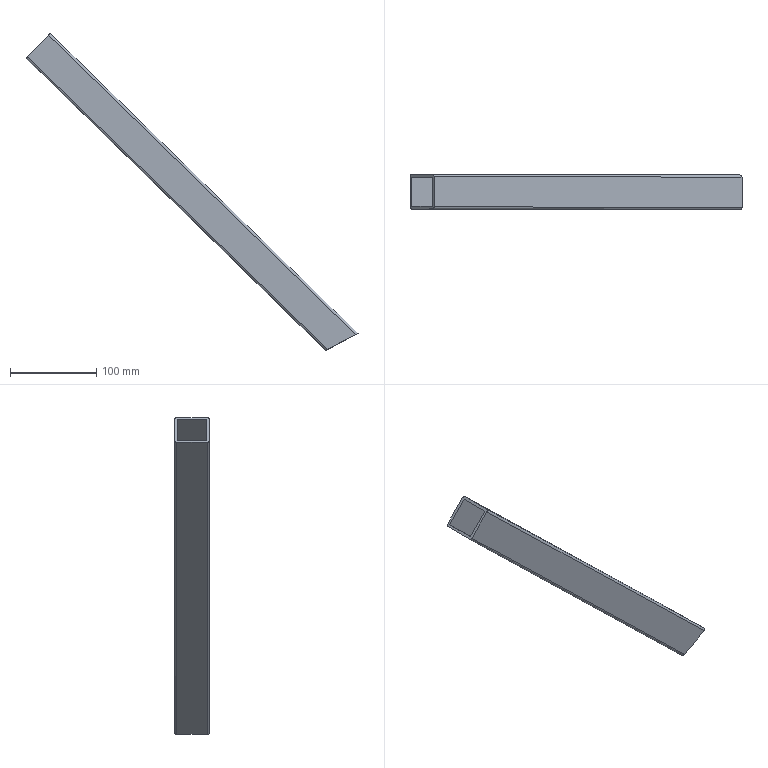Part | STEP file | SOLID | 1 solid | 14 faces | box 384.531 x 40 x 366.951 mm | volume 215519 mm3 | plane 10 | cylinder 4 | commonest cylinder face diameters 5 x4
STEP:
#1=CARTESIAN_POINT('',(0.,0.,0.));
#2=DIRECTION('',(0.,0.,1.));
#3=DIRECTION('',(1.,0.,0.));
#4=AXIS2_PLACEMENT_3D('',#1,#2,#3);
#5=CARTESIAN_POINT('',(1687.954,187.75,-2.424));
#6=VERTEX_POINT('',#5);
#7=CARTESIAN_POINT('',(1711.675,187.75,21.934));
#8=VERTEX_POINT('',#7);
#9=CARTESIAN_POINT('',(867.562,187.75,-844.86));
#10=DIRECTION('',(0.6977,0.,0.7164));
#11=VECTOR('',#10,1.);
#12=LINE('',#9,#11);
#13=CARTESIAN_POINT('',(0.,187.75,0.));
#14=DIRECTION('',(0.,1.,0.));
#15=DIRECTION('',(0.,0.,-1.));
#16=AXIS2_PLACEMENT_3D('',#13,#14,#15);
#17=PLANE('',#16);
#18=CARTESIAN_POINT('',(844.86,-867.562));
#19=DIRECTION('',(-0.7164,-0.6977));
#20=VECTOR('',#19,1.);
#21=LINE('',#18,#20);
#22=(GEOMETRIC_REPRESENTATION_CONTEXT(2)PARAMETRIC_REPRESENTATION_CONTEXT()REPRESENTATION_CONTEXT('',''));
#23=DEFINITIONAL_REPRESENTATION('',(#21),#22);
#24=PCURVE('',#17,#23);
#25=CARTESIAN_POINT('',(1685.861,150.75,-4.573));
#26=DIRECTION('',(-0.7164,0.,0.6977));
#27=DIRECTION('',(-0.6977,0.,-0.7164));
#28=AXIS2_PLACEMENT_3D('',#25,#26,#27);
#29=PLANE('',#28);
#30=CARTESIAN_POINT('',(1172.901,-37.));
#31=DIRECTION('',(-1.,0.));
#32=VECTOR('',#31,1.);
#33=LINE('',#30,#32);
#34=(GEOMETRIC_REPRESENTATION_CONTEXT(2)PARAMETRIC_REPRESENTATION_CONTEXT()REPRESENTATION_CONTEXT('',''));
#35=DEFINITIONAL_REPRESENTATION('',(#33),#34);
#36=PCURVE('',#29,#35);
#37=SURFACE_CURVE('',#12,(#24,#36),.PCURVE_S1.);
#38=EDGE_CURVE('',#6,#8,#37,.T.);
#39=ORIENTED_EDGE('',*,*,#38,.F.);
#40=CARTESIAN_POINT('',(2036.032,187.75,-341.393));
#41=VERTEX_POINT('',#40);
#42=CARTESIAN_POINT('',(2035.339,187.75,-340.718));
#43=DIRECTION('',(0.7164,0.,-0.6977));
#44=VECTOR('',#43,1.);
#45=LINE('',#42,#44);
#46=CARTESIAN_POINT('',(340.718,-2035.339));
#47=DIRECTION('',(0.6977,-0.7164));
#48=VECTOR('',#47,1.);
#49=LINE('',#46,#48);
#50=(GEOMETRIC_REPRESENTATION_CONTEXT(2)PARAMETRIC_REPRESENTATION_CONTEXT()REPRESENTATION_CONTEXT('',''));
#51=DEFINITIONAL_REPRESENTATION('',(#49),#50);
#52=PCURVE('',#17,#51);
#53=CARTESIAN_POINT('',(2035.339,150.75,-340.718));
#54=DIRECTION('',(-0.6977,0.,-0.7164));
#55=DIRECTION('',(0.7164,0.,-0.6977));
#56=AXIS2_PLACEMENT_3D('',#53,#54,#55);
#57=PLANE('',#56);
#58=CARTESIAN_POINT('',(0.,-37.));
#59=DIRECTION('',(1.,0.));
#60=VECTOR('',#59,1.);
#61=LINE('',#58,#60);
#62=(GEOMETRIC_REPRESENTATION_CONTEXT(2)PARAMETRIC_REPRESENTATION_CONTEXT()REPRESENTATION_CONTEXT('',''));
#63=DEFINITIONAL_REPRESENTATION('',(#61),#62);
#64=PCURVE('',#57,#63);
#65=SURFACE_CURVE('',#45,(#52,#64),.PCURVE_S1.);
#66=EDGE_CURVE('',#6,#41,#65,.T.);
#67=ORIENTED_EDGE('',*,*,#66,.T.);
#68=CARTESIAN_POINT('',(2067.606,187.75,-324.683));
#69=VERTEX_POINT('',#68);
#70=CARTESIAN_POINT('',(586.635,187.75,-1108.462));
#71=DIRECTION('',(-0.8839,0.,-0.4678));
#72=VECTOR('',#71,1.);
#73=LINE('',#70,#72);
#74=CARTESIAN_POINT('',(1108.462,-586.635));
#75=DIRECTION('',(0.4678,0.8839));
#76=VECTOR('',#75,1.);
#77=LINE('',#74,#76);
#78=(GEOMETRIC_REPRESENTATION_CONTEXT(2)PARAMETRIC_REPRESENTATION_CONTEXT()REPRESENTATION_CONTEXT('',''));
#79=DEFINITIONAL_REPRESENTATION('',(#77),#78);
#80=PCURVE('',#17,#79);
#81=CARTESIAN_POINT('',(2070.392,150.75,-323.209));
#82=DIRECTION('',(0.4678,0.,-0.8839));
#83=DIRECTION('',(0.8839,0.,0.4678));
#84=AXIS2_PLACEMENT_3D('',#81,#82,#83);
#85=PLANE('',#84);
#86=CARTESIAN_POINT('',(-1678.738,-37.));
#87=DIRECTION('',(-1.,0.));
#88=VECTOR('',#87,1.);
#89=LINE('',#86,#88);
#90=(GEOMETRIC_REPRESENTATION_CONTEXT(2)PARAMETRIC_REPRESENTATION_CONTEXT()REPRESENTATION_CONTEXT('',''));
#91=DEFINITIONAL_REPRESENTATION('',(#89),#90);
#92=PCURVE('',#85,#91);
#93=SURFACE_CURVE('',#73,(#80,#92),.PCURVE_S1.);
#94=EDGE_CURVE('',#69,#41,#93,.T.);
#95=ORIENTED_EDGE('',*,*,#94,.F.);
#96=CARTESIAN_POINT('',(1640.033,187.75,91.702));
#97=DIRECTION('',(-0.7164,0.,0.6977));
#98=VECTOR('',#97,1.);
#99=LINE('',#96,#98);
#100=CARTESIAN_POINT('',(-91.702,-1640.033));
#101=DIRECTION('',(-0.6977,0.7164));
#102=VECTOR('',#101,1.);
#103=LINE('',#100,#102);
#104=(GEOMETRIC_REPRESENTATION_CONTEXT(2)PARAMETRIC_REPRESENTATION_CONTEXT()REPRESENTATION_CONTEXT('',''));
#105=DEFINITIONAL_REPRESENTATION('',(#103),#104);
#106=PCURVE('',#17,#105);
#107=CARTESIAN_POINT('',(1640.033,150.75,91.702));
#108=DIRECTION('',(0.6977,0.,0.7164));
#109=DIRECTION('',(-0.7164,0.,0.6977));
#110=AXIS2_PLACEMENT_3D('',#107,#108,#109);
#111=PLANE('',#110);
#112=CARTESIAN_POINT('',(0.,-37.));
#113=DIRECTION('',(1.,0.));
#114=VECTOR('',#113,1.);
#115=LINE('',#112,#114);
#116=(GEOMETRIC_REPRESENTATION_CONTEXT(2)PARAMETRIC_REPRESENTATION_CONTEXT()REPRESENTATION_CONTEXT('',''));
#117=DEFINITIONAL_REPRESENTATION('',(#115),#116);
#118=PCURVE('',#111,#117);
#119=SURFACE_CURVE('',#99,(#106,#118),.PCURVE_S1.);
#120=EDGE_CURVE('',#69,#8,#119,.T.);
#121=ORIENTED_EDGE('',*,*,#120,.T.);
#122=EDGE_LOOP('',(#39,#67,#95,#121));
#123=FACE_BOUND('',#122,.T.);
#124=ADVANCED_FACE('',(#123),#17,.F.);
#125=CARTESIAN_POINT('',(2067.606,153.75,-324.683));
#126=VERTEX_POINT('',#125);
#127=CARTESIAN_POINT('',(2036.032,153.75,-341.393));
#128=VERTEX_POINT('',#127);
#129=CARTESIAN_POINT('',(586.635,153.75,-1108.462));
#130=DIRECTION('',(-0.8839,0.,-0.4678));
#131=VECTOR('',#130,1.);
#132=LINE('',#129,#131);
#133=CARTESIAN_POINT('',(0.,153.75,0.));
#134=DIRECTION('',(0.,1.,0.));
#135=DIRECTION('',(0.,0.,-1.));
#136=AXIS2_PLACEMENT_3D('',#133,#134,#135);
#137=PLANE('',#136);
#138=CARTESIAN_POINT('',(1108.462,-586.635));
#139=DIRECTION('',(0.4678,0.8839));
#140=VECTOR('',#139,1.);
#141=LINE('',#138,#140);
#142=(GEOMETRIC_REPRESENTATION_CONTEXT(2)PARAMETRIC_REPRESENTATION_CONTEXT()REPRESENTATION_CONTEXT('',''));
#143=DEFINITIONAL_REPRESENTATION('',(#141),#142);
#144=PCURVE('',#137,#143);
#145=CARTESIAN_POINT('',(-1678.738,-3.));
#146=DIRECTION('',(-1.,0.));
#147=VECTOR('',#146,1.);
#148=LINE('',#145,#147);
#149=(GEOMETRIC_REPRESENTATION_CONTEXT(2)PARAMETRIC_REPRESENTATION_CONTEXT()REPRESENTATION_CONTEXT('',''));
#150=DEFINITIONAL_REPRESENTATION('',(#148),#149);
#151=PCURVE('',#85,#150);
#152=SURFACE_CURVE('',#132,(#144,#151),.PCURVE_S1.);
#153=EDGE_CURVE('',#126,#128,#152,.T.);
#154=ORIENTED_EDGE('',*,*,#153,.T.);
#155=CARTESIAN_POINT('',(1687.954,153.75,-2.424));
#156=VERTEX_POINT('',#155);
#157=CARTESIAN_POINT('',(2035.339,153.75,-340.718));
#158=DIRECTION('',(0.7164,0.,-0.6977));
#159=VECTOR('',#158,1.);
#160=LINE('',#157,#159);
#161=CARTESIAN_POINT('',(340.718,-2035.339));
#162=DIRECTION('',(0.6977,-0.7164));
#163=VECTOR('',#162,1.);
#164=LINE('',#161,#163);
#165=(GEOMETRIC_REPRESENTATION_CONTEXT(2)PARAMETRIC_REPRESENTATION_CONTEXT()REPRESENTATION_CONTEXT('',''));
#166=DEFINITIONAL_REPRESENTATION('',(#164),#165);
#167=PCURVE('',#137,#166);
#168=CARTESIAN_POINT('',(0.,-3.));
#169=DIRECTION('',(1.,0.));
#170=VECTOR('',#169,1.);
#171=LINE('',#168,#170);
#172=(GEOMETRIC_REPRESENTATION_CONTEXT(2)PARAMETRIC_REPRESENTATION_CONTEXT()REPRESENTATION_CONTEXT('',''));
#173=DEFINITIONAL_REPRESENTATION('',(#171),#172);
#174=PCURVE('',#57,#173);
#175=SURFACE_CURVE('',#160,(#167,#174),.PCURVE_S1.);
#176=EDGE_CURVE('',#156,#128,#175,.T.);
#177=ORIENTED_EDGE('',*,*,#176,.F.);
#178=CARTESIAN_POINT('',(1711.675,153.75,21.934));
#179=VERTEX_POINT('',#178);
#180=CARTESIAN_POINT('',(867.562,153.75,-844.86));
#181=DIRECTION('',(0.6977,0.,0.7164));
#182=VECTOR('',#181,1.);
#183=LINE('',#180,#182);
#184=CARTESIAN_POINT('',(844.86,-867.562));
#185=DIRECTION('',(-0.7164,-0.6977));
#186=VECTOR('',#185,1.);
#187=LINE('',#184,#186);
#188=(GEOMETRIC_REPRESENTATION_CONTEXT(2)PARAMETRIC_REPRESENTATION_CONTEXT()REPRESENTATION_CONTEXT('',''));
#189=DEFINITIONAL_REPRESENTATION('',(#187),#188);
#190=PCURVE('',#137,#189);
#191=CARTESIAN_POINT('',(1172.901,-3.));
#192=DIRECTION('',(-1.,0.));
#193=VECTOR('',#192,1.);
#194=LINE('',#191,#193);
#195=(GEOMETRIC_REPRESENTATION_CONTEXT(2)PARAMETRIC_REPRESENTATION_CONTEXT()REPRESENTATION_CONTEXT('',''));
#196=DEFINITIONAL_REPRESENTATION('',(#194),#195);
#197=PCURVE('',#29,#196);
#198=SURFACE_CURVE('',#183,(#190,#197),.PCURVE_S1.);
#199=EDGE_CURVE('',#156,#179,#198,.T.);
#200=ORIENTED_EDGE('',*,*,#199,.T.);
#201=CARTESIAN_POINT('',(1640.033,153.75,91.702));
#202=DIRECTION('',(-0.7164,0.,0.6977));
#203=VECTOR('',#202,1.);
#204=LINE('',#201,#203);
#205=CARTESIAN_POINT('',(-91.702,-1640.033));
#206=DIRECTION('',(-0.6977,0.7164));
#207=VECTOR('',#206,1.);
#208=LINE('',#205,#207);
#209=(GEOMETRIC_REPRESENTATION_CONTEXT(2)PARAMETRIC_REPRESENTATION_CONTEXT()REPRESENTATION_CONTEXT('',''));
#210=DEFINITIONAL_REPRESENTATION('',(#208),#209);
#211=PCURVE('',#137,#210);
#212=CARTESIAN_POINT('',(0.,-3.));
#213=DIRECTION('',(1.,0.));
#214=VECTOR('',#213,1.);
#215=LINE('',#212,#214);
#216=(GEOMETRIC_REPRESENTATION_CONTEXT(2)PARAMETRIC_REPRESENTATION_CONTEXT()REPRESENTATION_CONTEXT('',''));
#217=DEFINITIONAL_REPRESENTATION('',(#215),#216);
#218=PCURVE('',#111,#217);
#219=SURFACE_CURVE('',#204,(#211,#218),.PCURVE_S1.);
#220=EDGE_CURVE('',#126,#179,#219,.T.);
#221=ORIENTED_EDGE('',*,*,#220,.F.);
#222=EDGE_LOOP('',(#154,#177,#200,#221));
#223=FACE_BOUND('',#222,.T.);
#224=ADVANCED_FACE('',(#223),#137,.T.);
#225=CARTESIAN_POINT('',(1711.675,150.75,21.934));
#226=DIRECTION('',(0.,1.,0.));
#227=VECTOR('',#226,1.);
#228=LINE('',#225,#227);
#229=CARTESIAN_POINT('',(-100.,0.));
#230=DIRECTION('',(0.,-1.));
#231=VECTOR('',#230,1.);
#232=LINE('',#229,#231);
#233=(GEOMETRIC_REPRESENTATION_CONTEXT(2)PARAMETRIC_REPRESENTATION_CONTEXT()REPRESENTATION_CONTEXT('',''));
#234=DEFINITIONAL_REPRESENTATION('',(#232),#233);
#235=PCURVE('',#111,#234);
#236=CARTESIAN_POINT('',(-37.,0.));
#237=DIRECTION('',(0.,-1.));
#238=VECTOR('',#237,1.);
#239=LINE('',#236,#238);
#240=(GEOMETRIC_REPRESENTATION_CONTEXT(2)PARAMETRIC_REPRESENTATION_CONTEXT()REPRESENTATION_CONTEXT('',''));
#241=DEFINITIONAL_REPRESENTATION('',(#239),#240);
#242=PCURVE('',#29,#241);
#243=SURFACE_CURVE('',#228,(#235,#242),.PCURVE_S1.);
#244=EDGE_CURVE('',#179,#8,#243,.T.);
#245=ORIENTED_EDGE('',*,*,#244,.T.);
#246=ORIENTED_EDGE('',*,*,#120,.F.);
#247=CARTESIAN_POINT('',(2067.606,150.75,-324.683));
#248=DIRECTION('',(0.,1.,0.));
#249=VECTOR('',#248,1.);
#250=LINE('',#247,#249);
#251=CARTESIAN_POINT('',(-596.821,0.));
#252=DIRECTION('',(0.,-1.));
#253=VECTOR('',#252,1.);
#254=LINE('',#251,#253);
#255=(GEOMETRIC_REPRESENTATION_CONTEXT(2)PARAMETRIC_REPRESENTATION_CONTEXT()REPRESENTATION_CONTEXT('',''));
#256=DEFINITIONAL_REPRESENTATION('',(#254),#255);
#257=PCURVE('',#111,#256);
#258=CARTESIAN_POINT('',(-3.152,0.));
#259=DIRECTION('',(0.,-1.));
#260=VECTOR('',#259,1.);
#261=LINE('',#258,#260);
#262=(GEOMETRIC_REPRESENTATION_CONTEXT(2)PARAMETRIC_REPRESENTATION_CONTEXT()REPRESENTATION_CONTEXT('',''));
#263=DEFINITIONAL_REPRESENTATION('',(#261),#262);
#264=PCURVE('',#85,#263);
#265=SURFACE_CURVE('',#250,(#257,#264),.PCURVE_S1.);
#266=EDGE_CURVE('',#126,#69,#265,.T.);
#267=ORIENTED_EDGE('',*,*,#266,.F.);
#268=ORIENTED_EDGE('',*,*,#220,.T.);
#269=EDGE_LOOP('',(#245,#246,#267,#268));
#270=FACE_BOUND('',#269,.T.);
#271=ADVANCED_FACE('',(#270),#111,.F.);
#272=CARTESIAN_POINT('',(2036.032,150.75,-341.393));
#273=DIRECTION('',(0.,1.,0.));
#274=VECTOR('',#273,1.);
#275=LINE('',#272,#274);
#276=CARTESIAN_POINT('',(0.9673,0.));
#277=DIRECTION('',(0.,-1.));
#278=VECTOR('',#277,1.);
#279=LINE('',#276,#278);
#280=(GEOMETRIC_REPRESENTATION_CONTEXT(2)PARAMETRIC_REPRESENTATION_CONTEXT()REPRESENTATION_CONTEXT('',''));
#281=DEFINITIONAL_REPRESENTATION('',(#279),#280);
#282=PCURVE('',#57,#281);
#283=CARTESIAN_POINT('',(-38.876,0.));
#284=DIRECTION('',(0.,-1.));
#285=VECTOR('',#284,1.);
#286=LINE('',#283,#285);
#287=(GEOMETRIC_REPRESENTATION_CONTEXT(2)PARAMETRIC_REPRESENTATION_CONTEXT()REPRESENTATION_CONTEXT('',''));
#288=DEFINITIONAL_REPRESENTATION('',(#286),#287);
#289=PCURVE('',#85,#288);
#290=SURFACE_CURVE('',#275,(#282,#289),.PCURVE_S1.);
#291=EDGE_CURVE('',#128,#41,#290,.T.);
#292=ORIENTED_EDGE('',*,*,#291,.T.);
#293=ORIENTED_EDGE('',*,*,#66,.F.);
#294=CARTESIAN_POINT('',(1687.954,150.75,-2.424));
#295=DIRECTION('',(0.,1.,0.));
#296=VECTOR('',#295,1.);
#297=LINE('',#294,#296);
#298=CARTESIAN_POINT('',(-484.891,0.));
#299=DIRECTION('',(0.,-1.));
#300=VECTOR('',#299,1.);
#301=LINE('',#298,#300);
#302=(GEOMETRIC_REPRESENTATION_CONTEXT(2)PARAMETRIC_REPRESENTATION_CONTEXT()REPRESENTATION_CONTEXT('',''));
#303=DEFINITIONAL_REPRESENTATION('',(#301),#302);
#304=PCURVE('',#57,#303);
#305=CARTESIAN_POINT('',(-3.,0.));
#306=DIRECTION('',(0.,-1.));
#307=VECTOR('',#306,1.);
#308=LINE('',#305,#307);
#309=(GEOMETRIC_REPRESENTATION_CONTEXT(2)PARAMETRIC_REPRESENTATION_CONTEXT()REPRESENTATION_CONTEXT('',''));
#310=DEFINITIONAL_REPRESENTATION('',(#308),#309);
#311=PCURVE('',#29,#310);
#312=SURFACE_CURVE('',#297,(#304,#311),.PCURVE_S1.);
#313=EDGE_CURVE('',#156,#6,#312,.T.);
#314=ORIENTED_EDGE('',*,*,#313,.F.);
#315=ORIENTED_EDGE('',*,*,#176,.T.);
#316=EDGE_LOOP('',(#292,#293,#314,#315));
#317=FACE_BOUND('',#316,.T.);
#318=ADVANCED_FACE('',(#317),#57,.F.);
#319=CARTESIAN_POINT('',(2033.246,188.25,-342.868));
#320=VERTEX_POINT('',#319);
#321=CARTESIAN_POINT('',(2035.568,190.75,-341.639));
#322=VERTEX_POINT('',#321);
#323=CARTESIAN_POINT('',(2035.568,188.25,-341.639));
#324=DIRECTION('',(0.4678,0.,-0.8839));
#325=DIRECTION('',(-0.8839,0.,-0.4678));
#326=AXIS2_PLACEMENT_3D('',#323,#324,#325);
#327=ELLIPSE('',#326,2.627,2.5);
#328=CARTESIAN_POINT('',(820.043,188.25,842.078));
#329=DIRECTION('',(-0.7164,0.,0.6977));
#330=DIRECTION('',(-0.6977,0.,-0.7164));
#331=AXIS2_PLACEMENT_3D('',#328,#329,#330);
#332=CYLINDRICAL_SURFACE('',#331,2.5);
#333=CARTESIAN_POINT('',(6.283,-1695.863));
#334=CARTESIAN_POINT('',(6.259,-1695.863));
#335=CARTESIAN_POINT('',(6.212,-1695.865));
#336=CARTESIAN_POINT('',(6.14,-1695.871));
#337=CARTESIAN_POINT('',(6.069,-1695.881));
#338=CARTESIAN_POINT('',(5.998,-1695.895));
#339=CARTESIAN_POINT('',(5.926,-1695.913));
#340=CARTESIAN_POINT('',(5.855,-1695.935));
#341=CARTESIAN_POINT('',(5.783,-1695.961));
#342=CARTESIAN_POINT('',(5.712,-1695.991));
#343=CARTESIAN_POINT('',(5.641,-1696.023));
#344=CARTESIAN_POINT('',(5.569,-1696.06));
#345=CARTESIAN_POINT('',(5.498,-1696.099));
#346=CARTESIAN_POINT('',(5.426,-1696.141));
#347=CARTESIAN_POINT('',(5.355,-1696.186));
#348=CARTESIAN_POINT('',(5.284,-1696.233));
#349=CARTESIAN_POINT('',(5.212,-1696.283));
#350=CARTESIAN_POINT('',(5.141,-1696.334));
#351=CARTESIAN_POINT('',(5.069,-1696.387));
#352=CARTESIAN_POINT('',(4.998,-1696.442));
#353=CARTESIAN_POINT('',(4.927,-1696.498));
#354=CARTESIAN_POINT('',(4.855,-1696.554));
#355=CARTESIAN_POINT('',(4.784,-1696.612));
#356=CARTESIAN_POINT('',(4.736,-1696.65));
#357=CARTESIAN_POINT('',(4.712,-1696.669));
#358=B_SPLINE_CURVE_WITH_KNOTS('',3,(#333,#334,#335,#336,#337,#338,#339,#340,#341,#342,#343,#344,#345,#346,#347,#348,#349,#350,#351,#352,#353,#354,#355,#356,#357),.UNSPECIFIED.,.F.,.F.,(4,1,1,1,1,1,1,1,1,1,1,1,1,1,1,1,1,1,1,1,1,1,4),(0.,0.0714,0.1428,0.2142,0.2856,0.357,0.4284,0.4998,0.5712,0.6426,0.714,0.7854,0.8568,0.9282,0.9996,1.071,1.142,1.214,1.285,1.357,1.428,1.499,1.571),.QUASI_UNIFORM_KNOTS.);
#359=(GEOMETRIC_REPRESENTATION_CONTEXT(2)PARAMETRIC_REPRESENTATION_CONTEXT()REPRESENTATION_CONTEXT('',''));
#360=DEFINITIONAL_REPRESENTATION('',(#358),#359);
#361=PCURVE('',#332,#360);
#362=CARTESIAN_POINT('',(-39.401,-37.5));
#363=DIRECTION('',(-1.,0.));
#364=AXIS2_PLACEMENT_2D('',#362,#363);
#365=ELLIPSE('',#364,2.627,2.5);
#366=(GEOMETRIC_REPRESENTATION_CONTEXT(2)PARAMETRIC_REPRESENTATION_CONTEXT()REPRESENTATION_CONTEXT('',''));
#367=DEFINITIONAL_REPRESENTATION('',(#365),#366);
#368=PCURVE('',#85,#367);
#369=SURFACE_CURVE('',#327,(#361,#368),.PCURVE_S1.);
#370=EDGE_CURVE('',#320,#322,#369,.T.);
#371=ORIENTED_EDGE('',*,*,#370,.F.);
#372=CARTESIAN_POINT('',(1685.861,188.25,-4.573));
#373=VERTEX_POINT('',#372);
#374=CARTESIAN_POINT('',(2033.246,188.25,-342.868));
#375=DIRECTION('',(0.7164,0.,-0.6977));
#376=VECTOR('',#375,1.);
#377=LINE('',#374,#376);
#378=CARTESIAN_POINT('',(6.283,-1695.863));
#379=DIRECTION('',(0.,-1.));
#380=VECTOR('',#379,1.);
#381=LINE('',#378,#380);
#382=(GEOMETRIC_REPRESENTATION_CONTEXT(2)PARAMETRIC_REPRESENTATION_CONTEXT()REPRESENTATION_CONTEXT('',''));
#383=DEFINITIONAL_REPRESENTATION('',(#381),#382);
#384=PCURVE('',#332,#383);
#385=CARTESIAN_POINT('',(2033.246,150.75,-342.868));
#386=DIRECTION('',(-0.6977,0.,-0.7164));
#387=DIRECTION('',(0.7164,0.,-0.6977));
#388=AXIS2_PLACEMENT_3D('',#385,#386,#387);
#389=PLANE('',#388);
#390=CARTESIAN_POINT('',(0.,-37.5));
#391=DIRECTION('',(1.,0.));
#392=VECTOR('',#391,1.);
#393=LINE('',#390,#392);
#394=(GEOMETRIC_REPRESENTATION_CONTEXT(2)PARAMETRIC_REPRESENTATION_CONTEXT()REPRESENTATION_CONTEXT('',''));
#395=DEFINITIONAL_REPRESENTATION('',(#393),#394);
#396=PCURVE('',#389,#395);
#397=SURFACE_CURVE('',#377,(#384,#396),.PCURVE_S1.);
#398=EDGE_CURVE('',#373,#320,#397,.T.);
#399=ORIENTED_EDGE('',*,*,#398,.F.);
#400=CARTESIAN_POINT('',(1687.606,190.75,-2.782));
#401=VERTEX_POINT('',#400);
#402=CARTESIAN_POINT('',(1687.606,188.25,-2.782));
#403=DIRECTION('',(-0.7164,0.,0.6977));
#404=DIRECTION('',(0.6977,0.,0.7164));
#405=AXIS2_PLACEMENT_3D('',#402,#403,#404);
#406=CIRCLE('',#405,2.5);
#407=CARTESIAN_POINT('',(3.142,-1210.972));
#408=DIRECTION('',(1.,0.));
#409=VECTOR('',#408,1.);
#410=LINE('',#407,#409);
#411=(GEOMETRIC_REPRESENTATION_CONTEXT(2)PARAMETRIC_REPRESENTATION_CONTEXT()REPRESENTATION_CONTEXT('',''));
#412=DEFINITIONAL_REPRESENTATION('',(#410),#411);
#413=PCURVE('',#332,#412);
#414=CARTESIAN_POINT('',(-2.5,-37.5));
#415=DIRECTION('',(-1.,0.));
#416=AXIS2_PLACEMENT_2D('',#414,#415);
#417=CIRCLE('',#416,2.5);
#418=(GEOMETRIC_REPRESENTATION_CONTEXT(2)PARAMETRIC_REPRESENTATION_CONTEXT()REPRESENTATION_CONTEXT('',''));
#419=DEFINITIONAL_REPRESENTATION('',(#417),#418);
#420=PCURVE('',#29,#419);
#421=SURFACE_CURVE('',#406,(#413,#420),.PCURVE_S1.);
#422=EDGE_CURVE('',#401,#373,#421,.T.);
#423=ORIENTED_EDGE('',*,*,#422,.F.);
#424=CARTESIAN_POINT('',(820.043,190.75,842.078));
#425=DIRECTION('',(-0.7164,0.,0.6977));
#426=VECTOR('',#425,1.);
#427=LINE('',#424,#426);
#428=CARTESIAN_POINT('',(4.712,0.));
#429=DIRECTION('',(0.,1.));
#430=VECTOR('',#429,1.);
#431=LINE('',#428,#430);
#432=(GEOMETRIC_REPRESENTATION_CONTEXT(2)PARAMETRIC_REPRESENTATION_CONTEXT()REPRESENTATION_CONTEXT('',''));
#433=DEFINITIONAL_REPRESENTATION('',(#431),#432);
#434=PCURVE('',#332,#433);
#435=CARTESIAN_POINT('',(0.,190.75,0.));
#436=DIRECTION('',(0.,1.,0.));
#437=DIRECTION('',(0.,0.,-1.));
#438=AXIS2_PLACEMENT_3D('',#435,#436,#437);
#439=PLANE('',#438);
#440=CARTESIAN_POINT('',(-842.078,-820.043));
#441=DIRECTION('',(-0.6977,0.7164));
#442=VECTOR('',#441,1.);
#443=LINE('',#440,#442);
#444=(GEOMETRIC_REPRESENTATION_CONTEXT(2)PARAMETRIC_REPRESENTATION_CONTEXT()REPRESENTATION_CONTEXT('',''));
#445=DEFINITIONAL_REPRESENTATION('',(#443),#444);
#446=PCURVE('',#439,#445);
#447=SURFACE_CURVE('',#427,(#434,#446),.PCURVE_S1.);
#448=EDGE_CURVE('',#322,#401,#447,.T.);
#449=ORIENTED_EDGE('',*,*,#448,.F.);
#450=EDGE_LOOP('',(#371,#399,#423,#449));
#451=FACE_BOUND('',#450,.T.);
#452=ADVANCED_FACE('',(#451),#332,.T.);
#453=CARTESIAN_POINT('',(2035.568,150.75,-341.639));
#454=VERTEX_POINT('',#453);
#455=CARTESIAN_POINT('',(2033.246,153.25,-342.868));
#456=VERTEX_POINT('',#455);
#457=CARTESIAN_POINT('',(2035.568,153.25,-341.639));
#458=DIRECTION('',(0.4678,0.,-0.8839));
#459=DIRECTION('',(0.8839,0.,0.4678));
#460=AXIS2_PLACEMENT_3D('',#457,#458,#459);
#461=ELLIPSE('',#460,2.627,2.5);
#462=CARTESIAN_POINT('',(2034.99,153.25,-341.077));
#463=DIRECTION('',(0.7164,0.,-0.6977));
#464=DIRECTION('',(0.6977,0.,0.7164));
#465=AXIS2_PLACEMENT_3D('',#462,#463,#464);
#466=CYLINDRICAL_SURFACE('',#465,2.5);
#467=CARTESIAN_POINT('',(1.571,0.806));
#468=CARTESIAN_POINT('',(1.595,0.7869));
#469=CARTESIAN_POINT('',(1.642,0.7485));
#470=CARTESIAN_POINT('',(1.714,0.6912));
#471=CARTESIAN_POINT('',(1.785,0.6346));
#472=CARTESIAN_POINT('',(1.856,0.5788));
#473=CARTESIAN_POINT('',(1.928,0.5241));
#474=CARTESIAN_POINT('',(1.999,0.4709));
#475=CARTESIAN_POINT('',(2.071,0.4194));
#476=CARTESIAN_POINT('',(2.142,0.3699));
#477=CARTESIAN_POINT('',(2.213,0.3226));
#478=CARTESIAN_POINT('',(2.285,0.2777));
#479=CARTESIAN_POINT('',(2.356,0.2356));
#480=CARTESIAN_POINT('',(2.428,0.1964));
#481=CARTESIAN_POINT('',(2.499,0.1602));
#482=CARTESIAN_POINT('',(2.57,0.1274));
#483=CARTESIAN_POINT('',(2.642,0.098));
#484=CARTESIAN_POINT('',(2.713,0.07222));
#485=CARTESIAN_POINT('',(2.785,0.05018));
#486=CARTESIAN_POINT('',(2.856,0.03199));
#487=CARTESIAN_POINT('',(2.927,0.01775));
#488=CARTESIAN_POINT('',(2.999,0.007526));
#489=CARTESIAN_POINT('',(3.07,0.001371));
#490=CARTESIAN_POINT('',(3.118,-0.000001738));
#491=CARTESIAN_POINT('',(3.142,0.));
#492=B_SPLINE_CURVE_WITH_KNOTS('',3,(#467,#468,#469,#470,#471,#472,#473,#474,#475,#476,#477,#478,#479,#480,#481,#482,#483,#484,#485,#486,#487,#488,#489,#490,#491),.UNSPECIFIED.,.F.,.F.,(4,1,1,1,1,1,1,1,1,1,1,1,1,1,1,1,1,1,1,1,1,1,4),(1.571,1.642,1.714,1.785,1.856,1.928,1.999,2.071,2.142,2.213,2.285,2.356,2.428,2.499,2.57,2.642,2.713,2.785,2.856,2.927,2.999,3.07,3.142),.QUASI_UNIFORM_KNOTS.);
#493=(GEOMETRIC_REPRESENTATION_CONTEXT(2)PARAMETRIC_REPRESENTATION_CONTEXT()REPRESENTATION_CONTEXT('',''));
#494=DEFINITIONAL_REPRESENTATION('',(#492),#493);
#495=PCURVE('',#466,#494);
#496=CARTESIAN_POINT('',(-39.401,-2.5));
#497=DIRECTION('',(1.,0.));
#498=AXIS2_PLACEMENT_2D('',#496,#497);
#499=ELLIPSE('',#498,2.627,2.5);
#500=(GEOMETRIC_REPRESENTATION_CONTEXT(2)PARAMETRIC_REPRESENTATION_CONTEXT()REPRESENTATION_CONTEXT('',''));
#501=DEFINITIONAL_REPRESENTATION('',(#499),#500);
#502=PCURVE('',#85,#501);
#503=SURFACE_CURVE('',#461,(#495,#502),.PCURVE_S1.);
#504=EDGE_CURVE('',#454,#456,#503,.T.);
#505=ORIENTED_EDGE('',*,*,#504,.F.);
#506=CARTESIAN_POINT('',(1687.606,150.75,-2.782));
#507=VERTEX_POINT('',#506);
#508=CARTESIAN_POINT('',(2034.99,150.75,-341.077));
#509=DIRECTION('',(0.7164,0.,-0.6977));
#510=VECTOR('',#509,1.);
#511=LINE('',#508,#510);
#512=CARTESIAN_POINT('',(1.571,0.));
#513=DIRECTION('',(0.,1.));
#514=VECTOR('',#513,1.);
#515=LINE('',#512,#514);
#516=(GEOMETRIC_REPRESENTATION_CONTEXT(2)PARAMETRIC_REPRESENTATION_CONTEXT()REPRESENTATION_CONTEXT('',''));
#517=DEFINITIONAL_REPRESENTATION('',(#515),#516);
#518=PCURVE('',#466,#517);
#519=CARTESIAN_POINT('',(0.,150.75,0.));
#520=DIRECTION('',(0.,1.,0.));
#521=DIRECTION('',(0.,0.,-1.));
#522=AXIS2_PLACEMENT_3D('',#519,#520,#521);
#523=PLANE('',#522);
#524=CARTESIAN_POINT('',(341.077,-2034.99));
#525=DIRECTION('',(0.6977,-0.7164));
#526=VECTOR('',#525,1.);
#527=LINE('',#524,#526);
#528=(GEOMETRIC_REPRESENTATION_CONTEXT(2)PARAMETRIC_REPRESENTATION_CONTEXT()REPRESENTATION_CONTEXT('',''));
#529=DEFINITIONAL_REPRESENTATION('',(#527),#528);
#530=PCURVE('',#523,#529);
#531=SURFACE_CURVE('',#511,(#518,#530),.PCURVE_S1.);
#532=EDGE_CURVE('',#507,#454,#531,.T.);
#533=ORIENTED_EDGE('',*,*,#532,.F.);
#534=CARTESIAN_POINT('',(1685.861,153.25,-4.573));
#535=VERTEX_POINT('',#534);
#536=CARTESIAN_POINT('',(1687.606,153.25,-2.782));
#537=DIRECTION('',(-0.7164,0.,0.6977));
#538=DIRECTION('',(0.6977,0.,0.7164));
#539=AXIS2_PLACEMENT_3D('',#536,#537,#538);
#540=CIRCLE('',#539,2.5);
#541=CARTESIAN_POINT('',(6.283,-484.891));
#542=DIRECTION('',(-1.,0.));
#543=VECTOR('',#542,1.);
#544=LINE('',#541,#543);
#545=(GEOMETRIC_REPRESENTATION_CONTEXT(2)PARAMETRIC_REPRESENTATION_CONTEXT()REPRESENTATION_CONTEXT('',''));
#546=DEFINITIONAL_REPRESENTATION('',(#544),#545);
#547=PCURVE('',#466,#546);
#548=CARTESIAN_POINT('',(-2.5,-2.5));
#549=DIRECTION('',(-1.,0.));
#550=AXIS2_PLACEMENT_2D('',#548,#549);
#551=CIRCLE('',#550,2.5);
#552=(GEOMETRIC_REPRESENTATION_CONTEXT(2)PARAMETRIC_REPRESENTATION_CONTEXT()REPRESENTATION_CONTEXT('',''));
#553=DEFINITIONAL_REPRESENTATION('',(#551),#552);
#554=PCURVE('',#29,#553);
#555=SURFACE_CURVE('',#540,(#547,#554),.PCURVE_S1.);
#556=EDGE_CURVE('',#535,#507,#555,.T.);
#557=ORIENTED_EDGE('',*,*,#556,.F.);
#558=CARTESIAN_POINT('',(1614.22,153.25,65.194));
#559=DIRECTION('',(-0.7164,0.,0.6977));
#560=VECTOR('',#559,1.);
#561=LINE('',#558,#560);
#562=CARTESIAN_POINT('',(3.142,-584.891));
#563=DIRECTION('',(0.,-1.));
#564=VECTOR('',#563,1.);
#565=LINE('',#562,#564);
#566=(GEOMETRIC_REPRESENTATION_CONTEXT(2)PARAMETRIC_REPRESENTATION_CONTEXT()REPRESENTATION_CONTEXT('',''));
#567=DEFINITIONAL_REPRESENTATION('',(#565),#566);
#568=PCURVE('',#466,#567);
#569=CARTESIAN_POINT('',(-584.891,-2.5));
#570=DIRECTION('',(-1.,0.));
#571=VECTOR('',#570,1.);
#572=LINE('',#569,#571);
#573=(GEOMETRIC_REPRESENTATION_CONTEXT(2)PARAMETRIC_REPRESENTATION_CONTEXT()REPRESENTATION_CONTEXT('',''));
#574=DEFINITIONAL_REPRESENTATION('',(#572),#573);
#575=PCURVE('',#389,#574);
#576=SURFACE_CURVE('',#561,(#568,#575),.PCURVE_S1.);
#577=EDGE_CURVE('',#456,#535,#576,.T.);
#578=ORIENTED_EDGE('',*,*,#577,.F.);
#579=EDGE_LOOP('',(#505,#533,#557,#578));
#580=FACE_BOUND('',#579,.T.);
#581=ADVANCED_FACE('',(#580),#466,.T.);
#582=CARTESIAN_POINT('',(1713.768,188.25,24.084));
#583=VERTEX_POINT('',#582);
#584=CARTESIAN_POINT('',(1712.024,190.75,22.293));
#585=VERTEX_POINT('',#584);
#586=CARTESIAN_POINT('',(1712.024,188.25,22.293));
#587=DIRECTION('',(-0.7164,0.,0.6977));
#588=DIRECTION('',(0.6977,0.,0.7164));
#589=AXIS2_PLACEMENT_3D('',#586,#587,#588);
#590=CIRCLE('',#589,2.5);
#591=CARTESIAN_POINT('',(844.462,188.25,867.153));
#592=DIRECTION('',(0.7164,0.,-0.6977));
#593=DIRECTION('',(0.6977,0.,0.7164));
#594=AXIS2_PLACEMENT_3D('',#591,#592,#593);
#595=CYLINDRICAL_SURFACE('',#594,2.5);
#596=CARTESIAN_POINT('',(6.283,1210.972));
#597=DIRECTION('',(-1.,0.));
#598=VECTOR('',#597,1.);
#599=LINE('',#596,#598);
#600=(GEOMETRIC_REPRESENTATION_CONTEXT(2)PARAMETRIC_REPRESENTATION_CONTEXT()REPRESENTATION_CONTEXT('',''));
#601=DEFINITIONAL_REPRESENTATION('',(#599),#600);
#602=PCURVE('',#595,#601);
#603=CARTESIAN_POINT('',(-37.5,-37.5));
#604=DIRECTION('',(-1.,0.));
#605=AXIS2_PLACEMENT_2D('',#603,#604);
#606=CIRCLE('',#605,2.5);
#607=(GEOMETRIC_REPRESENTATION_CONTEXT(2)PARAMETRIC_REPRESENTATION_CONTEXT()REPRESENTATION_CONTEXT('',''));
#608=DEFINITIONAL_REPRESENTATION('',(#606),#607);
#609=PCURVE('',#29,#608);
#610=SURFACE_CURVE('',#590,(#602,#609),.PCURVE_S1.);
#611=EDGE_CURVE('',#583,#585,#610,.T.);
#612=ORIENTED_EDGE('',*,*,#611,.F.);
#613=CARTESIAN_POINT('',(2070.392,188.25,-323.209));
#614=VERTEX_POINT('',#613);
#615=CARTESIAN_POINT('',(1642.126,188.25,93.851));
#616=DIRECTION('',(-0.7164,0.,0.6977));
#617=VECTOR('',#616,1.);
#618=LINE('',#615,#617);
#619=CARTESIAN_POINT('',(6.283,1110.972));
#620=DIRECTION('',(0.,-1.));
#621=VECTOR('',#620,1.);
#622=LINE('',#619,#621);
#623=(GEOMETRIC_REPRESENTATION_CONTEXT(2)PARAMETRIC_REPRESENTATION_CONTEXT()REPRESENTATION_CONTEXT('',''));
#624=DEFINITIONAL_REPRESENTATION('',(#622),#623);
#625=PCURVE('',#595,#624);
#626=CARTESIAN_POINT('',(1642.126,150.75,93.851));
#627=DIRECTION('',(0.6977,0.,0.7164));
#628=DIRECTION('',(-0.7164,0.,0.6977));
#629=AXIS2_PLACEMENT_3D('',#626,#627,#628);
#630=PLANE('',#629);
#631=CARTESIAN_POINT('',(0.,-37.5));
#632=DIRECTION('',(1.,0.));
#633=VECTOR('',#632,1.);
#634=LINE('',#631,#633);
#635=(GEOMETRIC_REPRESENTATION_CONTEXT(2)PARAMETRIC_REPRESENTATION_CONTEXT()REPRESENTATION_CONTEXT('',''));
#636=DEFINITIONAL_REPRESENTATION('',(#634),#635);
#637=PCURVE('',#630,#636);
#638=SURFACE_CURVE('',#618,(#625,#637),.PCURVE_S1.);
#639=EDGE_CURVE('',#614,#583,#638,.T.);
#640=ORIENTED_EDGE('',*,*,#639,.F.);
#641=CARTESIAN_POINT('',(2068.071,190.75,-324.437));
#642=VERTEX_POINT('',#641);
#643=CARTESIAN_POINT('',(2068.071,188.25,-324.437));
#644=DIRECTION('',(0.4678,0.,-0.8839));
#645=DIRECTION('',(0.8839,0.,0.4678));
#646=AXIS2_PLACEMENT_3D('',#643,#644,#645);
#647=ELLIPSE('',#646,2.627,2.5);
#648=CARTESIAN_POINT('',(4.712,1707.954));
#649=CARTESIAN_POINT('',(4.736,1707.973));
#650=CARTESIAN_POINT('',(4.784,1708.012));
#651=CARTESIAN_POINT('',(4.855,1708.069));
#652=CARTESIAN_POINT('',(4.927,1708.125));
#653=CARTESIAN_POINT('',(4.998,1708.181));
#654=CARTESIAN_POINT('',(5.069,1708.236));
#655=CARTESIAN_POINT('',(5.141,1708.289));
#656=CARTESIAN_POINT('',(5.212,1708.341));
#657=CARTESIAN_POINT('',(5.284,1708.39));
#658=CARTESIAN_POINT('',(5.355,1708.437));
#659=CARTESIAN_POINT('',(5.426,1708.482));
#660=CARTESIAN_POINT('',(5.498,1708.524));
#661=CARTESIAN_POINT('',(5.569,1708.564));
#662=CARTESIAN_POINT('',(5.641,1708.6));
#663=CARTESIAN_POINT('',(5.712,1708.633));
#664=CARTESIAN_POINT('',(5.783,1708.662));
#665=CARTESIAN_POINT('',(5.855,1708.688));
#666=CARTESIAN_POINT('',(5.926,1708.71));
#667=CARTESIAN_POINT('',(5.998,1708.728));
#668=CARTESIAN_POINT('',(6.069,1708.742));
#669=CARTESIAN_POINT('',(6.14,1708.752));
#670=CARTESIAN_POINT('',(6.212,1708.759));
#671=CARTESIAN_POINT('',(6.259,1708.76));
#672=CARTESIAN_POINT('',(6.283,1708.76));
#673=B_SPLINE_CURVE_WITH_KNOTS('',3,(#648,#649,#650,#651,#652,#653,#654,#655,#656,#657,#658,#659,#660,#661,#662,#663,#664,#665,#666,#667,#668,#669,#670,#671,#672),.UNSPECIFIED.,.F.,.F.,(4,1,1,1,1,1,1,1,1,1,1,1,1,1,1,1,1,1,1,1,1,1,4),(4.712,4.784,4.855,4.927,4.998,5.069,5.141,5.212,5.284,5.355,5.426,5.498,5.569,5.641,5.712,5.783,5.855,5.926,5.998,6.069,6.14,6.212,6.283),.QUASI_UNIFORM_KNOTS.);
#674=(GEOMETRIC_REPRESENTATION_CONTEXT(2)PARAMETRIC_REPRESENTATION_CONTEXT()REPRESENTATION_CONTEXT('',''));
#675=DEFINITIONAL_REPRESENTATION('',(#673),#674);
#676=PCURVE('',#595,#675);
#677=CARTESIAN_POINT('',(-2.627,-37.5));
#678=DIRECTION('',(1.,0.));
#679=AXIS2_PLACEMENT_2D('',#677,#678);
#680=ELLIPSE('',#679,2.627,2.5);
#681=(GEOMETRIC_REPRESENTATION_CONTEXT(2)PARAMETRIC_REPRESENTATION_CONTEXT()REPRESENTATION_CONTEXT('',''));
#682=DEFINITIONAL_REPRESENTATION('',(#680),#681);
#683=PCURVE('',#85,#682);
#684=SURFACE_CURVE('',#647,(#676,#683),.PCURVE_S1.);
#685=EDGE_CURVE('',#642,#614,#684,.T.);
#686=ORIENTED_EDGE('',*,*,#685,.F.);
#687=CARTESIAN_POINT('',(844.462,190.75,867.153));
#688=DIRECTION('',(0.7164,0.,-0.6977));
#689=VECTOR('',#688,1.);
#690=LINE('',#687,#689);
#691=CARTESIAN_POINT('',(4.712,0.));
#692=DIRECTION('',(0.,1.));
#693=VECTOR('',#692,1.);
#694=LINE('',#691,#693);
#695=(GEOMETRIC_REPRESENTATION_CONTEXT(2)PARAMETRIC_REPRESENTATION_CONTEXT()REPRESENTATION_CONTEXT('',''));
#696=DEFINITIONAL_REPRESENTATION('',(#694),#695);
#697=PCURVE('',#595,#696);
#698=CARTESIAN_POINT('',(-867.153,-844.462));
#699=DIRECTION('',(0.6977,-0.7164));
#700=VECTOR('',#699,1.);
#701=LINE('',#698,#700);
#702=(GEOMETRIC_REPRESENTATION_CONTEXT(2)PARAMETRIC_REPRESENTATION_CONTEXT()REPRESENTATION_CONTEXT('',''));
#703=DEFINITIONAL_REPRESENTATION('',(#701),#702);
#704=PCURVE('',#439,#703);
#705=SURFACE_CURVE('',#690,(#697,#704),.PCURVE_S1.);
#706=EDGE_CURVE('',#585,#642,#705,.T.);
#707=ORIENTED_EDGE('',*,*,#706,.F.);
#708=EDGE_LOOP('',(#612,#640,#686,#707));
#709=FACE_BOUND('',#708,.T.);
#710=ADVANCED_FACE('',(#709),#595,.T.);
#711=CARTESIAN_POINT('',(1712.024,150.75,22.293));
#712=VERTEX_POINT('',#711);
#713=CARTESIAN_POINT('',(1713.768,153.25,24.084));
#714=VERTEX_POINT('',#713);
#715=CARTESIAN_POINT('',(1712.024,153.25,22.293));
#716=DIRECTION('',(-0.7164,0.,0.6977));
#717=DIRECTION('',(0.6977,0.,0.7164));
#718=AXIS2_PLACEMENT_3D('',#715,#716,#717);
#719=CIRCLE('',#718,2.5);
#720=CARTESIAN_POINT('',(1640.382,153.25,92.06));
#721=DIRECTION('',(-0.7164,0.,0.6977));
#722=DIRECTION('',(-0.6977,0.,-0.7164));
#723=AXIS2_PLACEMENT_3D('',#720,#721,#722);
#724=CYLINDRICAL_SURFACE('',#723,2.5);
#725=CARTESIAN_POINT('',(-3.142,-100.));
#726=DIRECTION('',(1.,0.));
#727=VECTOR('',#726,1.);
#728=LINE('',#725,#727);
#729=(GEOMETRIC_REPRESENTATION_CONTEXT(2)PARAMETRIC_REPRESENTATION_CONTEXT()REPRESENTATION_CONTEXT('',''));
#730=DEFINITIONAL_REPRESENTATION('',(#728),#729);
#731=PCURVE('',#724,#730);
#732=CARTESIAN_POINT('',(-37.5,-2.5));
#733=DIRECTION('',(-1.,0.));
#734=AXIS2_PLACEMENT_2D('',#732,#733);
#735=CIRCLE('',#734,2.5);
#736=(GEOMETRIC_REPRESENTATION_CONTEXT(2)PARAMETRIC_REPRESENTATION_CONTEXT()REPRESENTATION_CONTEXT('',''));
#737=DEFINITIONAL_REPRESENTATION('',(#735),#736);
#738=PCURVE('',#29,#737);
#739=SURFACE_CURVE('',#719,(#731,#738),.PCURVE_S1.);
#740=EDGE_CURVE('',#712,#714,#739,.T.);
#741=ORIENTED_EDGE('',*,*,#740,.F.);
#742=CARTESIAN_POINT('',(2068.071,150.75,-324.437));
#743=VERTEX_POINT('',#742);
#744=CARTESIAN_POINT('',(1640.382,150.75,92.06));
#745=DIRECTION('',(-0.7164,0.,0.6977));
#746=VECTOR('',#745,1.);
#747=LINE('',#744,#746);
#748=CARTESIAN_POINT('',(1.571,0.));
#749=DIRECTION('',(0.,1.));
#750=VECTOR('',#749,1.);
#751=LINE('',#748,#750);
#752=(GEOMETRIC_REPRESENTATION_CONTEXT(2)PARAMETRIC_REPRESENTATION_CONTEXT()REPRESENTATION_CONTEXT('',''));
#753=DEFINITIONAL_REPRESENTATION('',(#751),#752);
#754=PCURVE('',#724,#753);
#755=CARTESIAN_POINT('',(-92.06,-1640.382));
#756=DIRECTION('',(-0.6977,0.7164));
#757=VECTOR('',#756,1.);
#758=LINE('',#755,#757);
#759=(GEOMETRIC_REPRESENTATION_CONTEXT(2)PARAMETRIC_REPRESENTATION_CONTEXT()REPRESENTATION_CONTEXT('',''));
#760=DEFINITIONAL_REPRESENTATION('',(#758),#759);
#761=PCURVE('',#523,#760);
#762=SURFACE_CURVE('',#747,(#754,#761),.PCURVE_S1.);
#763=EDGE_CURVE('',#743,#712,#762,.T.);
#764=ORIENTED_EDGE('',*,*,#763,.F.);
#765=CARTESIAN_POINT('',(2070.392,153.25,-323.209));
#766=VERTEX_POINT('',#765);
#767=CARTESIAN_POINT('',(2068.071,153.25,-324.437));
#768=DIRECTION('',(0.4678,0.,-0.8839));
#769=DIRECTION('',(-0.8839,0.,-0.4678));
#770=AXIS2_PLACEMENT_3D('',#767,#768,#769);
#771=ELLIPSE('',#770,2.627,2.5);
#772=CARTESIAN_POINT('',(3.142,-597.788));
#773=CARTESIAN_POINT('',(3.118,-597.788));
#774=CARTESIAN_POINT('',(3.07,-597.786));
#775=CARTESIAN_POINT('',(2.999,-597.78));
#776=CARTESIAN_POINT('',(2.927,-597.77));
#777=CARTESIAN_POINT('',(2.856,-597.756));
#778=CARTESIAN_POINT('',(2.785,-597.738));
#779=CARTESIAN_POINT('',(2.713,-597.716));
#780=CARTESIAN_POINT('',(2.642,-597.69));
#781=CARTESIAN_POINT('',(2.57,-597.66));
#782=CARTESIAN_POINT('',(2.499,-597.628));
#783=CARTESIAN_POINT('',(2.428,-597.591));
#784=CARTESIAN_POINT('',(2.356,-597.552));
#785=CARTESIAN_POINT('',(2.285,-597.51));
#786=CARTESIAN_POINT('',(2.213,-597.465));
#787=CARTESIAN_POINT('',(2.142,-597.418));
#788=CARTESIAN_POINT('',(2.071,-597.368));
#789=CARTESIAN_POINT('',(1.999,-597.317));
#790=CARTESIAN_POINT('',(1.928,-597.264));
#791=CARTESIAN_POINT('',(1.856,-597.209));
#792=CARTESIAN_POINT('',(1.785,-597.153));
#793=CARTESIAN_POINT('',(1.714,-597.097));
#794=CARTESIAN_POINT('',(1.642,-597.039));
#795=CARTESIAN_POINT('',(1.595,-597.001));
#796=CARTESIAN_POINT('',(1.571,-596.982));
#797=B_SPLINE_CURVE_WITH_KNOTS('',3,(#772,#773,#774,#775,#776,#777,#778,#779,#780,#781,#782,#783,#784,#785,#786,#787,#788,#789,#790,#791,#792,#793,#794,#795,#796),.UNSPECIFIED.,.F.,.F.,(4,1,1,1,1,1,1,1,1,1,1,1,1,1,1,1,1,1,1,1,1,1,4),(3.142,3.213,3.284,3.356,3.427,3.499,3.57,3.641,3.713,3.784,3.856,3.927,3.998,4.07,4.141,4.213,4.284,4.355,4.427,4.498,4.57,4.641,4.712),.QUASI_UNIFORM_KNOTS.);
#798=(GEOMETRIC_REPRESENTATION_CONTEXT(2)PARAMETRIC_REPRESENTATION_CONTEXT()REPRESENTATION_CONTEXT('',''));
#799=DEFINITIONAL_REPRESENTATION('',(#797),#798);
#800=PCURVE('',#724,#799);
#801=CARTESIAN_POINT('',(-2.627,-2.5));
#802=DIRECTION('',(-1.,0.));
#803=AXIS2_PLACEMENT_2D('',#801,#802);
#804=ELLIPSE('',#803,2.627,2.5);
#805=(GEOMETRIC_REPRESENTATION_CONTEXT(2)PARAMETRIC_REPRESENTATION_CONTEXT()REPRESENTATION_CONTEXT('',''));
#806=DEFINITIONAL_REPRESENTATION('',(#804),#805);
#807=PCURVE('',#85,#806);
#808=SURFACE_CURVE('',#771,(#800,#807),.PCURVE_S1.);
#809=EDGE_CURVE('',#766,#743,#808,.T.);
#810=ORIENTED_EDGE('',*,*,#809,.F.);
#811=CARTESIAN_POINT('',(2070.392,153.25,-323.209));
#812=DIRECTION('',(0.7164,0.,-0.6977));
#813=VECTOR('',#812,1.);
#814=LINE('',#811,#813);
#815=CARTESIAN_POINT('',(3.142,-597.788));
#816=DIRECTION('',(0.,-1.));
#817=VECTOR('',#816,1.);
#818=LINE('',#815,#817);
#819=(GEOMETRIC_REPRESENTATION_CONTEXT(2)PARAMETRIC_REPRESENTATION_CONTEXT()REPRESENTATION_CONTEXT('',''));
#820=DEFINITIONAL_REPRESENTATION('',(#818),#819);
#821=PCURVE('',#724,#820);
#822=CARTESIAN_POINT('',(-597.788,-2.5));
#823=DIRECTION('',(-1.,0.));
#824=VECTOR('',#823,1.);
#825=LINE('',#822,#824);
#826=(GEOMETRIC_REPRESENTATION_CONTEXT(2)PARAMETRIC_REPRESENTATION_CONTEXT()REPRESENTATION_CONTEXT('',''));
#827=DEFINITIONAL_REPRESENTATION('',(#825),#826);
#828=PCURVE('',#630,#827);
#829=SURFACE_CURVE('',#814,(#821,#828),.PCURVE_S1.);
#830=EDGE_CURVE('',#714,#766,#829,.T.);
#831=ORIENTED_EDGE('',*,*,#830,.F.);
#832=EDGE_LOOP('',(#741,#764,#810,#831));
#833=FACE_BOUND('',#832,.T.);
#834=ADVANCED_FACE('',(#833),#724,.T.);
#835=CARTESIAN_POINT('',(1685.861,190.75,-4.573));
#836=DIRECTION('',(0.6977,0.,0.7164));
#837=VECTOR('',#836,1.);
#838=LINE('',#835,#837);
#839=CARTESIAN_POINT('',(4.573,-1685.861));
#840=DIRECTION('',(-0.7164,-0.6977));
#841=VECTOR('',#840,1.);
#842=LINE('',#839,#841);
#843=(GEOMETRIC_REPRESENTATION_CONTEXT(2)PARAMETRIC_REPRESENTATION_CONTEXT()REPRESENTATION_CONTEXT('',''));
#844=DEFINITIONAL_REPRESENTATION('',(#842),#843);
#845=PCURVE('',#439,#844);
#846=CARTESIAN_POINT('',(0.,-40.));
#847=DIRECTION('',(-1.,0.));
#848=VECTOR('',#847,1.);
#849=LINE('',#846,#848);
#850=(GEOMETRIC_REPRESENTATION_CONTEXT(2)PARAMETRIC_REPRESENTATION_CONTEXT()REPRESENTATION_CONTEXT('',''));
#851=DEFINITIONAL_REPRESENTATION('',(#849),#850);
#852=PCURVE('',#29,#851);
#853=SURFACE_CURVE('',#838,(#845,#852),.PCURVE_S1.);
#854=EDGE_CURVE('',#401,#585,#853,.T.);
#855=ORIENTED_EDGE('',*,*,#854,.T.);
#856=ORIENTED_EDGE('',*,*,#706,.T.);
#857=CARTESIAN_POINT('',(2070.392,190.75,-323.209));
#858=DIRECTION('',(-0.8839,0.,-0.4678));
#859=VECTOR('',#858,1.);
#860=LINE('',#857,#859);
#861=CARTESIAN_POINT('',(323.209,-2070.392));
#862=DIRECTION('',(0.4678,0.8839));
#863=VECTOR('',#862,1.);
#864=LINE('',#861,#863);
#865=(GEOMETRIC_REPRESENTATION_CONTEXT(2)PARAMETRIC_REPRESENTATION_CONTEXT()REPRESENTATION_CONTEXT('',''));
#866=DEFINITIONAL_REPRESENTATION('',(#864),#865);
#867=PCURVE('',#439,#866);
#868=CARTESIAN_POINT('',(0.,-40.));
#869=DIRECTION('',(-1.,0.));
#870=VECTOR('',#869,1.);
#871=LINE('',#868,#870);
#872=(GEOMETRIC_REPRESENTATION_CONTEXT(2)PARAMETRIC_REPRESENTATION_CONTEXT()REPRESENTATION_CONTEXT('',''));
#873=DEFINITIONAL_REPRESENTATION('',(#871),#872);
#874=PCURVE('',#85,#873);
#875=SURFACE_CURVE('',#860,(#867,#874),.PCURVE_S1.);
#876=EDGE_CURVE('',#642,#322,#875,.T.);
#877=ORIENTED_EDGE('',*,*,#876,.T.);
#878=ORIENTED_EDGE('',*,*,#448,.T.);
#879=EDGE_LOOP('',(#855,#856,#877,#878));
#880=FACE_BOUND('',#879,.T.);
#881=ADVANCED_FACE('',(#880),#439,.T.);
#882=CARTESIAN_POINT('',(2070.392,150.75,-323.209));
#883=DIRECTION('',(-0.8839,0.,-0.4678));
#884=VECTOR('',#883,1.);
#885=LINE('',#882,#884);
#886=CARTESIAN_POINT('',(323.209,-2070.392));
#887=DIRECTION('',(0.4678,0.8839));
#888=VECTOR('',#887,1.);
#889=LINE('',#886,#888);
#890=(GEOMETRIC_REPRESENTATION_CONTEXT(2)PARAMETRIC_REPRESENTATION_CONTEXT()REPRESENTATION_CONTEXT('',''));
#891=DEFINITIONAL_REPRESENTATION('',(#889),#890);
#892=PCURVE('',#523,#891);
#893=CARTESIAN_POINT('',(0.,0.));
#894=DIRECTION('',(-1.,0.));
#895=VECTOR('',#894,1.);
#896=LINE('',#893,#895);
#897=(GEOMETRIC_REPRESENTATION_CONTEXT(2)PARAMETRIC_REPRESENTATION_CONTEXT()REPRESENTATION_CONTEXT('',''));
#898=DEFINITIONAL_REPRESENTATION('',(#896),#897);
#899=PCURVE('',#85,#898);
#900=SURFACE_CURVE('',#885,(#892,#899),.PCURVE_S1.);
#901=EDGE_CURVE('',#743,#454,#900,.T.);
#902=ORIENTED_EDGE('',*,*,#901,.F.);
#903=ORIENTED_EDGE('',*,*,#763,.T.);
#904=CARTESIAN_POINT('',(1685.861,150.75,-4.573));
#905=DIRECTION('',(0.6977,0.,0.7164));
#906=VECTOR('',#905,1.);
#907=LINE('',#904,#906);
#908=CARTESIAN_POINT('',(4.573,-1685.861));
#909=DIRECTION('',(-0.7164,-0.6977));
#910=VECTOR('',#909,1.);
#911=LINE('',#908,#910);
#912=(GEOMETRIC_REPRESENTATION_CONTEXT(2)PARAMETRIC_REPRESENTATION_CONTEXT()REPRESENTATION_CONTEXT('',''));
#913=DEFINITIONAL_REPRESENTATION('',(#911),#912);
#914=PCURVE('',#523,#913);
#915=CARTESIAN_POINT('',(0.,0.));
#916=DIRECTION('',(-1.,0.));
#917=VECTOR('',#916,1.);
#918=LINE('',#915,#917);
#919=(GEOMETRIC_REPRESENTATION_CONTEXT(2)PARAMETRIC_REPRESENTATION_CONTEXT()REPRESENTATION_CONTEXT('',''));
#920=DEFINITIONAL_REPRESENTATION('',(#918),#919);
#921=PCURVE('',#29,#920);
#922=SURFACE_CURVE('',#907,(#914,#921),.PCURVE_S1.);
#923=EDGE_CURVE('',#507,#712,#922,.T.);
#924=ORIENTED_EDGE('',*,*,#923,.F.);
#925=ORIENTED_EDGE('',*,*,#532,.T.);
#926=EDGE_LOOP('',(#902,#903,#924,#925));
#927=FACE_BOUND('',#926,.T.);
#928=ADVANCED_FACE('',(#927),#523,.F.);
#929=CARTESIAN_POINT('',(1713.768,150.75,24.084));
#930=DIRECTION('',(0.,1.,0.));
#931=VECTOR('',#930,1.);
#932=LINE('',#929,#931);
#933=CARTESIAN_POINT('',(-100.,0.));
#934=DIRECTION('',(0.,-1.));
#935=VECTOR('',#934,1.);
#936=LINE('',#933,#935);
#937=(GEOMETRIC_REPRESENTATION_CONTEXT(2)PARAMETRIC_REPRESENTATION_CONTEXT()REPRESENTATION_CONTEXT('',''));
#938=DEFINITIONAL_REPRESENTATION('',(#936),#937);
#939=PCURVE('',#630,#938);
#940=CARTESIAN_POINT('',(-40.,0.));
#941=DIRECTION('',(0.,-1.));
#942=VECTOR('',#941,1.);
#943=LINE('',#940,#942);
#944=(GEOMETRIC_REPRESENTATION_CONTEXT(2)PARAMETRIC_REPRESENTATION_CONTEXT()REPRESENTATION_CONTEXT('',''));
#945=DEFINITIONAL_REPRESENTATION('',(#943),#944);
#946=PCURVE('',#29,#945);
#947=SURFACE_CURVE('',#932,(#939,#946),.PCURVE_S1.);
#948=EDGE_CURVE('',#714,#583,#947,.T.);
#949=ORIENTED_EDGE('',*,*,#948,.F.);
#950=ORIENTED_EDGE('',*,*,#830,.T.);
#951=CARTESIAN_POINT('',(2070.392,150.75,-323.209));
#952=DIRECTION('',(0.,1.,0.));
#953=VECTOR('',#952,1.);
#954=LINE('',#951,#953);
#955=CARTESIAN_POINT('',(-597.788,0.));
#956=DIRECTION('',(0.,-1.));
#957=VECTOR('',#956,1.);
#958=LINE('',#955,#957);
#959=(GEOMETRIC_REPRESENTATION_CONTEXT(2)PARAMETRIC_REPRESENTATION_CONTEXT()REPRESENTATION_CONTEXT('',''));
#960=DEFINITIONAL_REPRESENTATION('',(#958),#959);
#961=PCURVE('',#630,#960);
#962=CARTESIAN_POINT('',(0.,0.));
#963=DIRECTION('',(0.,-1.));
#964=VECTOR('',#963,1.);
#965=LINE('',#962,#964);
#966=(GEOMETRIC_REPRESENTATION_CONTEXT(2)PARAMETRIC_REPRESENTATION_CONTEXT()REPRESENTATION_CONTEXT('',''));
#967=DEFINITIONAL_REPRESENTATION('',(#965),#966);
#968=PCURVE('',#85,#967);
#969=SURFACE_CURVE('',#954,(#961,#968),.PCURVE_S1.);
#970=EDGE_CURVE('',#766,#614,#969,.T.);
#971=ORIENTED_EDGE('',*,*,#970,.T.);
#972=ORIENTED_EDGE('',*,*,#639,.T.);
#973=EDGE_LOOP('',(#949,#950,#971,#972));
#974=FACE_BOUND('',#973,.T.);
#975=ADVANCED_FACE('',(#974),#630,.T.);
#976=ORIENTED_EDGE('',*,*,#923,.T.);
#977=ORIENTED_EDGE('',*,*,#740,.T.);
#978=ORIENTED_EDGE('',*,*,#948,.T.);
#979=ORIENTED_EDGE('',*,*,#611,.T.);
#980=ORIENTED_EDGE('',*,*,#854,.F.);
#981=ORIENTED_EDGE('',*,*,#422,.T.);
#982=CARTESIAN_POINT('',(1685.861,150.75,-4.573));
#983=DIRECTION('',(0.,1.,0.));
#984=VECTOR('',#983,1.);
#985=LINE('',#982,#984);
#986=CARTESIAN_POINT('',(0.,0.));
#987=DIRECTION('',(0.,-1.));
#988=VECTOR('',#987,1.);
#989=LINE('',#986,#988);
#990=(GEOMETRIC_REPRESENTATION_CONTEXT(2)PARAMETRIC_REPRESENTATION_CONTEXT()REPRESENTATION_CONTEXT('',''));
#991=DEFINITIONAL_REPRESENTATION('',(#989),#990);
#992=PCURVE('',#29,#991);
#993=CARTESIAN_POINT('',(-484.891,0.));
#994=DIRECTION('',(0.,-1.));
#995=VECTOR('',#994,1.);
#996=LINE('',#993,#995);
#997=(GEOMETRIC_REPRESENTATION_CONTEXT(2)PARAMETRIC_REPRESENTATION_CONTEXT()REPRESENTATION_CONTEXT('',''));
#998=DEFINITIONAL_REPRESENTATION('',(#996),#997);
#999=PCURVE('',#389,#998);
#1000=SURFACE_CURVE('',#985,(#992,#999),.PCURVE_S1.);
#1001=EDGE_CURVE('',#535,#373,#1000,.T.);
#1002=ORIENTED_EDGE('',*,*,#1001,.F.);
#1003=ORIENTED_EDGE('',*,*,#556,.T.);
#1004=EDGE_LOOP('',(#976,#977,#978,#979,#980,#981,#1002,#1003));
#1005=FACE_BOUND('',#1004,.T.);
#1006=ORIENTED_EDGE('',*,*,#199,.F.);
#1007=ORIENTED_EDGE('',*,*,#313,.T.);
#1008=ORIENTED_EDGE('',*,*,#38,.T.);
#1009=ORIENTED_EDGE('',*,*,#244,.F.);
#1010=EDGE_LOOP('',(#1006,#1007,#1008,#1009));
#1011=FACE_BOUND('',#1010,.T.);
#1012=ADVANCED_FACE('',(#1005,#1011),#29,.T.);
#1013=CARTESIAN_POINT('',(2033.246,150.75,-342.868));
#1014=DIRECTION('',(0.,1.,0.));
#1015=VECTOR('',#1014,1.);
#1016=LINE('',#1013,#1015);
#1017=CARTESIAN_POINT('',(0.,0.));
#1018=DIRECTION('',(0.,-1.));
#1019=VECTOR('',#1018,1.);
#1020=LINE('',#1017,#1019);
#1021=(GEOMETRIC_REPRESENTATION_CONTEXT(2)PARAMETRIC_REPRESENTATION_CONTEXT()REPRESENTATION_CONTEXT('',''));
#1022=DEFINITIONAL_REPRESENTATION('',(#1020),#1021);
#1023=PCURVE('',#389,#1022);
#1024=CARTESIAN_POINT('',(-42.028,0.));
#1025=DIRECTION('',(0.,-1.));
#1026=VECTOR('',#1025,1.);
#1027=LINE('',#1024,#1026);
#1028=(GEOMETRIC_REPRESENTATION_CONTEXT(2)PARAMETRIC_REPRESENTATION_CONTEXT()REPRESENTATION_CONTEXT('',''));
#1029=DEFINITIONAL_REPRESENTATION('',(#1027),#1028);
#1030=PCURVE('',#85,#1029);
#1031=SURFACE_CURVE('',#1016,(#1023,#1030),.PCURVE_S1.);
#1032=EDGE_CURVE('',#456,#320,#1031,.T.);
#1033=ORIENTED_EDGE('',*,*,#1032,.F.);
#1034=ORIENTED_EDGE('',*,*,#577,.T.);
#1035=ORIENTED_EDGE('',*,*,#1001,.T.);
#1036=ORIENTED_EDGE('',*,*,#398,.T.);
#1037=EDGE_LOOP('',(#1033,#1034,#1035,#1036));
#1038=FACE_BOUND('',#1037,.T.);
#1039=ADVANCED_FACE('',(#1038),#389,.T.);
#1040=ORIENTED_EDGE('',*,*,#153,.F.);
#1041=ORIENTED_EDGE('',*,*,#266,.T.);
#1042=ORIENTED_EDGE('',*,*,#94,.T.);
#1043=ORIENTED_EDGE('',*,*,#291,.F.);
#1044=EDGE_LOOP('',(#1040,#1041,#1042,#1043));
#1045=FACE_BOUND('',#1044,.T.);
#1046=ORIENTED_EDGE('',*,*,#970,.F.);
#1047=ORIENTED_EDGE('',*,*,#809,.T.);
#1048=ORIENTED_EDGE('',*,*,#901,.T.);
#1049=ORIENTED_EDGE('',*,*,#504,.T.);
#1050=ORIENTED_EDGE('',*,*,#1032,.T.);
#1051=ORIENTED_EDGE('',*,*,#370,.T.);
#1052=ORIENTED_EDGE('',*,*,#876,.F.);
#1053=ORIENTED_EDGE('',*,*,#685,.T.);
#1054=EDGE_LOOP('',(#1046,#1047,#1048,#1049,#1050,#1051,#1052,#1053));
#1055=FACE_BOUND('',#1054,.T.);
#1056=ADVANCED_FACE('',(#1045,#1055),#85,.T.);
#1057=CLOSED_SHELL('',(#124,#224,#271,#318,#452,#581,#710,#834,#881,#928,#975,#1012,#1039,#1056));
#1058=MANIFOLD_SOLID_BREP('',#1057);
#1059=(LENGTH_UNIT()NAMED_UNIT(*)SI_UNIT(.MILLI.,.METRE.));
#1060=UNCERTAINTY_MEASURE_WITH_UNIT(LENGTH_MEASURE(0.0000001),#1059,'','');
#1061=(NAMED_UNIT(*)PLANE_ANGLE_UNIT()SI_UNIT($,.RADIAN.));
#1062=(NAMED_UNIT(*)SI_UNIT($,.STERADIAN.)SOLID_ANGLE_UNIT());
#1063=(GEOMETRIC_REPRESENTATION_CONTEXT(3)GLOBAL_UNCERTAINTY_ASSIGNED_CONTEXT((#1060))GLOBAL_UNIT_ASSIGNED_CONTEXT((#1059,#1061,#1062))REPRESENTATION_CONTEXT('',''));
#1064=ADVANCED_BREP_SHAPE_REPRESENTATION('',(#4,#1058),#1063);